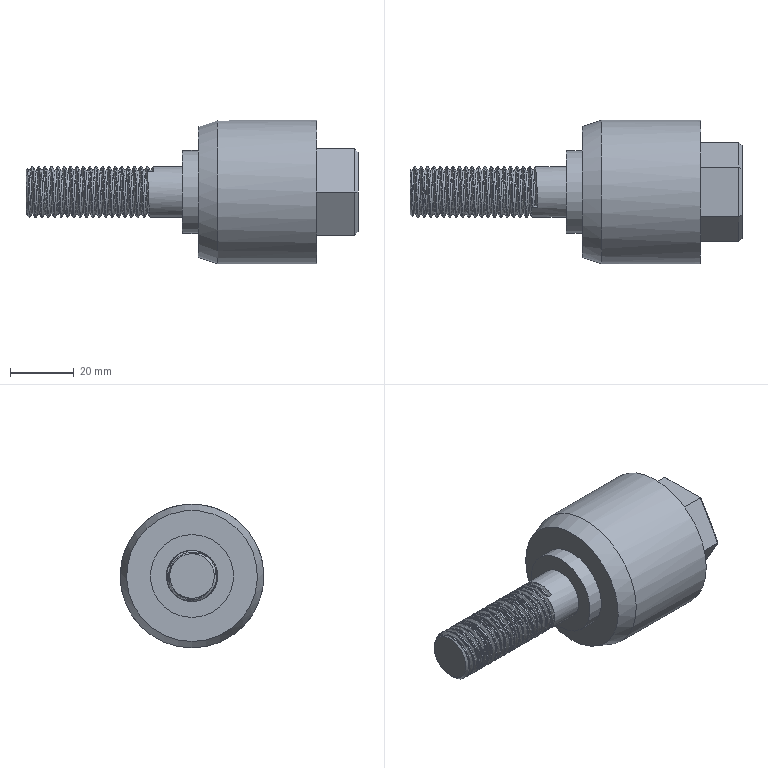Part | STEP file | Tube feed_id558_x_t | 1 solid | 45 faces | box 104 x 45 x 45 mm | volume 77621 mm3 | cylinder 23 | plane 18 | cone 2 | spline 2 | commonest cylinder face diameters 16 x20 14 x1 26 x1 45 x1